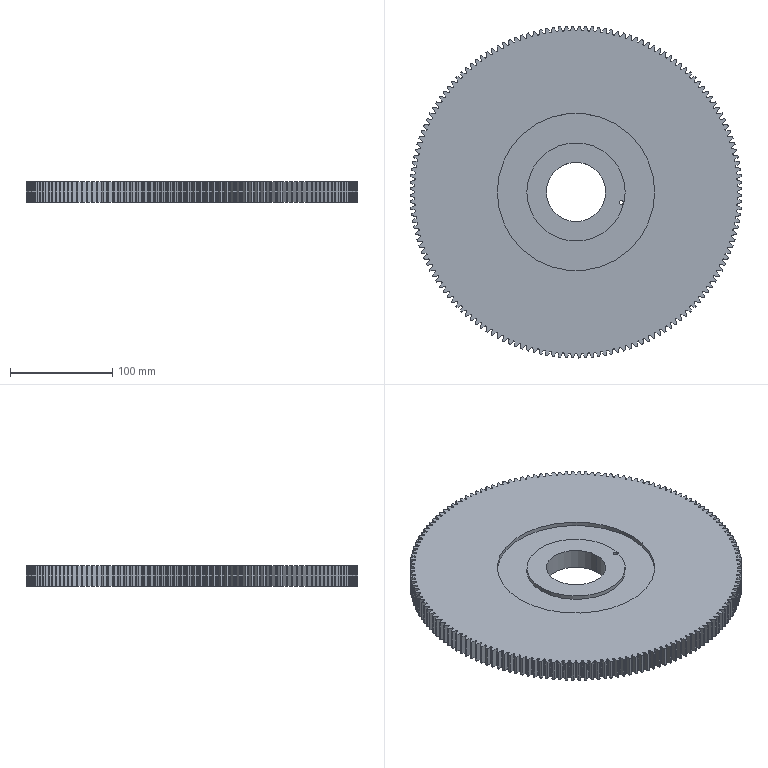Part | SolidWorks | features ICE 5, Cut 1, Extrusion 1 | 1 solid | 1043 faces | box 323.966 x 323.966 x 20 mm | volume 1463021 mm3 | cylinder 717 | spline 320 | plane 6 | commonest cylinder face diameters 1.52 x384 315 x161 324 x160 96 x4 153.6 x4 4 x2